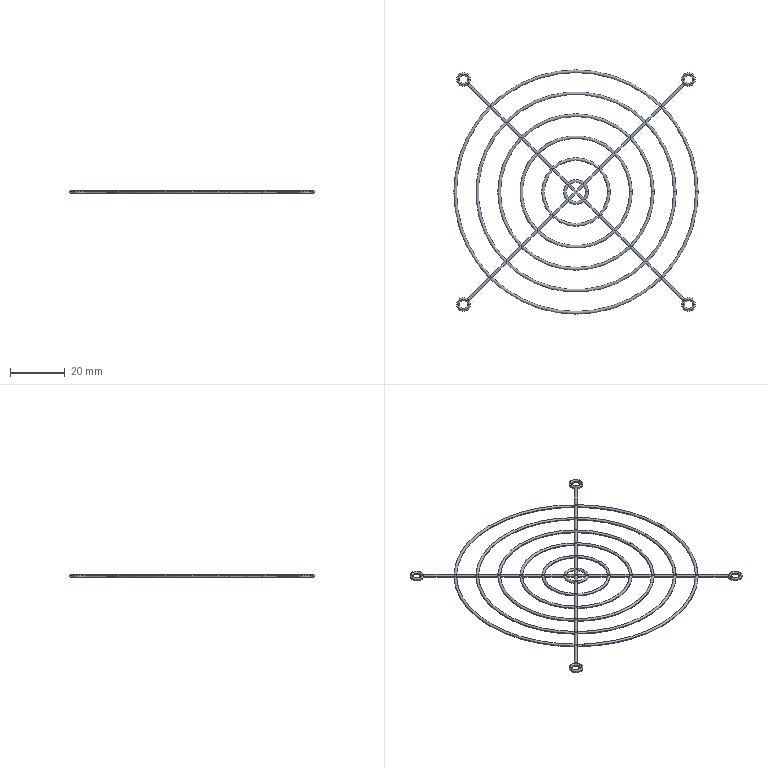Part | SolidWorks | features Fillet 4, ICE 3, Extrusion 1, Revolution 1 | 1 solid | 160 faces | box 89 x 89 x 1 mm | volume 913.094 mm3 | cylinder 80 | torus 76 | plane 4 | commonest cylinder face diameters 1 x56 5 x16 3 x8